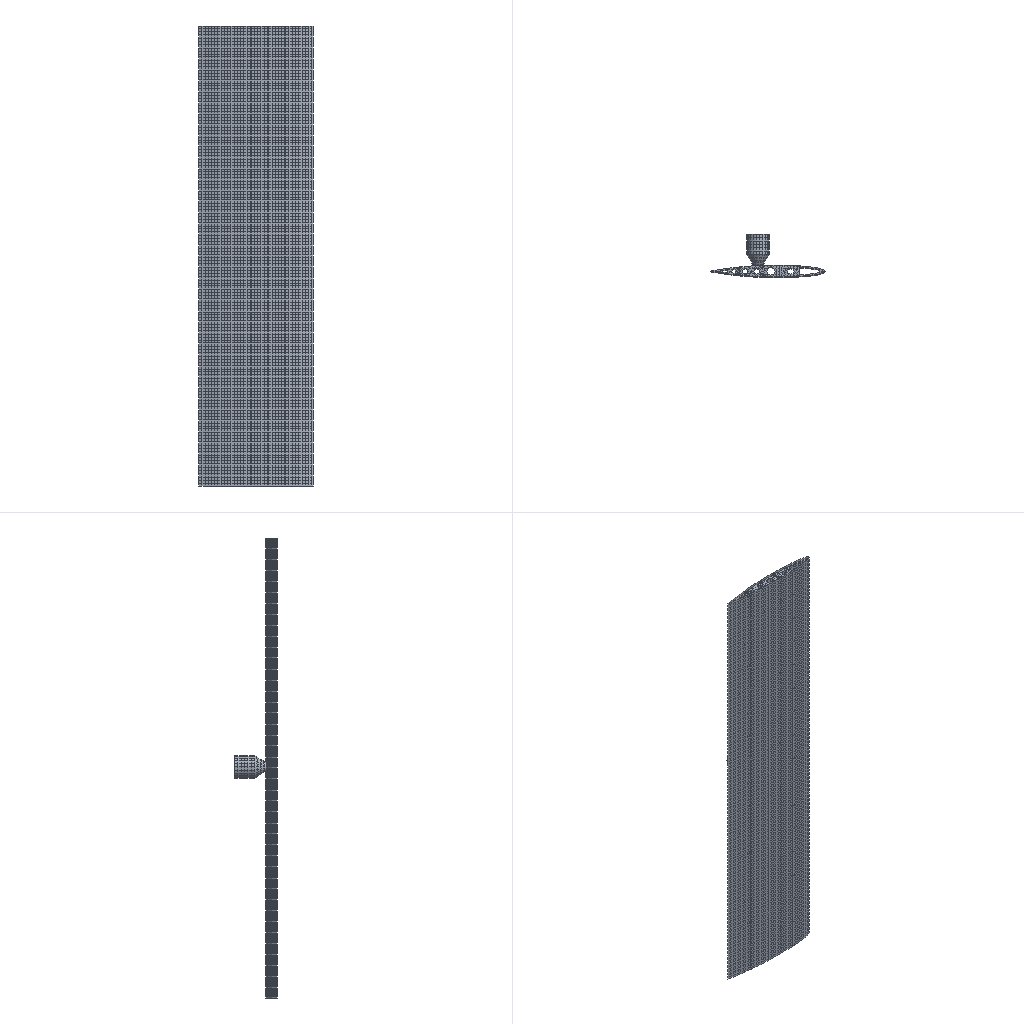Simulation study | abaqus
Set-up summary:
category,name,step,type,value,unit,region
solver,abaqus
solver,version,,,Abaqus/Explicit 2020
units,not stated in the deck,,not stated
analysis,deck,,transient,transient
load_step,Step-1,Step-1,transient,nlgeom=True
contact,interactions,,,general=0 pairs=1 ties=0
load_step,requested,,,1
mesh,nodes,,,18102
mesh,elements,,,18515
element_type,S3,,shell,954
element_type,S4R,,shell,17011
element_type,C3D8R,,solid,550
load,load commands in deck,,count,1
bc,support commands in deck,,count,6
material,MATERIAL-1,,in results
check,setup vs results,,match,"per instance, exact: element labels, types and connectivity; labels of the nodes the elements use; coordinates of those nodes at SINGLE_PRECISION in 2 of 2 instance(s)"
Abaqus input file, long lists of numbers shortened:
*Heading
** Job name: Job-1 Model name: Model-1
** Generated by: Abaqus/CAE 2020
*Preprint, echo=NO, model=NO, history=NO, contact=NO
**
** PARTS
**
*Part, name=w-1
*Node
      1,   3.41,   45.098,        4020.
      2,   3.41,   45.098,        4000.
** (17362 more lines like these left out)
*Element, type=S4R
1,    1,    2, 1571, 1573
2, 1573, 1571,    3,    5
** (17009 more lines like these left out)
*Element, type=S3
13119, 14626,   861,  1609
13120, 14627,  1606,  1605
** (952 more lines like these left out)
*Nset, nset=Set-1, generate
     1,  17364,      1
*Elset, elset=Set-1, generate
     1,  17965,      1
** Section: Section-1
*Shell Section, elset=Set-1, material=Material-1
0.5, 5
*End Part
**
*Part, name=w-2
*Node
      1,   -91.551,   323.76,   2048.173
      2,  -103.375,   323.76,   2074.064
** (735 more lines like these left out)
*Element, type=C3D8R
  1,  91,  84,  83, 123,  24,  17,  16,  56
  2, 123, 124,  92, 115,  56,  57,  25,  48
** (548 more lines like these left out)
*Node
    738,       -187.5,   323.76,        2020.
*Nset, nset=w-2-RefPt_, internal
738,
*Nset, nset=Set-1, generate
   1,  737,    1
*Elset, elset=Set-1, generate
   1,  550,    1
*Nset, nset=Set-2, generate
   1,  737,    1
*Elset, elset=Set-2, generate
   1,  550,    1
** Section: Section-2
*Solid Section, elset=Set-2, material=Material-1
,
*End Part
**
**
** ASSEMBLY
**
*Assembly, name=Assembly
**
*Instance, name=w-1-1, part=w-1
*End Instance
**
*Instance, name=w-2-1, part=w-2
*End Instance
**
*Nset, nset=Set-1, instance=w-1-1
     1,     2,     3,     4,     5,     6,     7,     8,    12,    13,    14,    15,    16,    17,    21,    22
    23,    24,    25,    26,    27,    28,    29,    30,    31,    32,    33,    34,    35,    38,    39,    40
** (53 more lines like these left out)
*Elset, elset=Set-1, instance=w-1-1
     1,     2,     3,     4,     5,    14,    15,    16,    17,    18,    19,    20,    21,    22,    23,    24
    25,    26,    27,    28,    29,    30,    31,    32,    33,    34,    35,    36,    37,    38,   179,   180
** (56 more lines like these left out)
*Nset, nset=Set-2, instance=w-2-1
 738,
*Nset, nset=Set-3, instance=w-2-1
 738,
*Nset, nset=b_Set-4, instance=w-2-1, generate
   1,  737,    1
*Elset, elset=b_Set-4, instance=w-2-1, generate
   1,  550,    1
*Nset, nset=_PickedSet14, internal, instance=w-2-1
 738,
*Elset, elset=_m_Surf-1_S2, internal, instance=w-2-1, generate
  1,  55,   1
*Elset, elset=_m_Surf-1_S4, internal, instance=w-2-1
   1,  11,  13,  18,  19,  21,  22,  23,  25,  26,  28,  30,  33,  48,  49,  50
  51,  56,  66,  68,  73,  74,  76,  77,  78,  80,  81,  83,  85,  88, 103, 104
** (9 more lines like these left out)
*Elset, elset=_m_Surf-1_S6, internal, instance=w-2-1
   3,   4,  12,  58,  59,  67, 113, 114, 122, 168, 169, 177, 223, 224, 232, 278
 279, 287, 333, 334, 342, 388, 389, 397, 443, 444, 452, 498, 499, 507
*Elset, elset=_m_Surf-1_S3, internal, instance=w-2-1, generate
  24,  519,   55
*Elset, elset=_m_Surf-1_S5, internal, instance=w-2-1, generate
  29,  524,   55
*Elset, elset=_m_Surf-1_S1, internal, instance=w-2-1, generate
 496,  550,    1
*Surface, type=ELEMENT, name=m_Surf-1
_m_Surf-1_S2, S2
_m_Surf-1_S4, S4
_m_Surf-1_S6, S6
_m_Surf-1_S3, S3
_m_Surf-1_S5, S5
_m_Surf-1_S1, S1
*Elset, elset=_s_Surf-1_SNEG, internal, instance=w-1-1
    14,    15,    16,    17,    18,    19,    20,    21,    22,    23,    24,    25,    26,    27,    28,    29
    30,    31,    32,    33,    34,    35,    36,    37,    38,    39,    40,    41,    42,    43,    44,    45
** (723 more lines like these left out)
*Surface, type=ELEMENT, name=s_Surf-1
_s_Surf-1_SNEG, SNEG
** Constraint: Constraint-1
*Rigid Body, ref node=_PickedSet14, elset=b_Set-4
*End Assembly
**
** MATERIALS
**
*Material, name=Material-1
*Density
 2.7e-09,
*Elastic
72000., 0.28
**
** INTERACTION PROPERTIES
**
*Surface Interaction, name=IntProp-1
*Friction
 0.2,
*Surface Behavior, pressure-overclosure=HARD
**
** PREDEFINED FIELDS
**
** Name: Predefined Field-1   Type: Velocity
*Initial Conditions, type=VELOCITY
Set-2, 1, 0.
Set-2, 2, -5000.
Set-2, 3, 0.
** ----------------------------------------------------------------
**
** STEP: Step-1
**
*Step, name=Step-1, nlgeom=YES
*Dynamic, Explicit
, 0.01
*Bulk Viscosity
0.06, 1.2
** Mass Scaling: Semi-Automatic
**               Whole Model
*Fixed Mass Scaling, factor=50.
**
** BOUNDARY CONDITIONS
**
** Name: BC-1 Type: 对称/反对称/完全固定
*Boundary
Set-1, ENCASTRE
** Name: BC-2 Type: 位移/转角
*Boundary
Set-3, 1, 1
Set-3, 3, 3
Set-3, 4, 4
Set-3, 5, 5
Set-3, 6, 6
**
** INTERACTIONS
**
** Interaction: Int-1
*Contact Pair, interaction=IntProp-1, mechanical constraint=KINEMATIC, cpset=Int-1
m_Surf-1, s_Surf-1
**
** OUTPUT REQUESTS
**
*Restart, write, number interval=1, time marks=NO
**
** FIELD OUTPUT: F-Output-1
**
*Output, field, variable=PRESELECT
**
** HISTORY OUTPUT: H-Output-1
**
*Output, history, variable=PRESELECT
*End Step
Results summary:
result,step,Step-1,completed,increments=5480 time=0.01/0.01
result,analysis,,,transient
result,last_loadstep,,,1
result,analysis steps,,count,1
result,primary field,,,"U, UR"
result,reaction total,,FX,-2828.759,model units
result,reaction total,,FY,-1007.165,model units
result,reaction total,,FZ,1460.787,model units